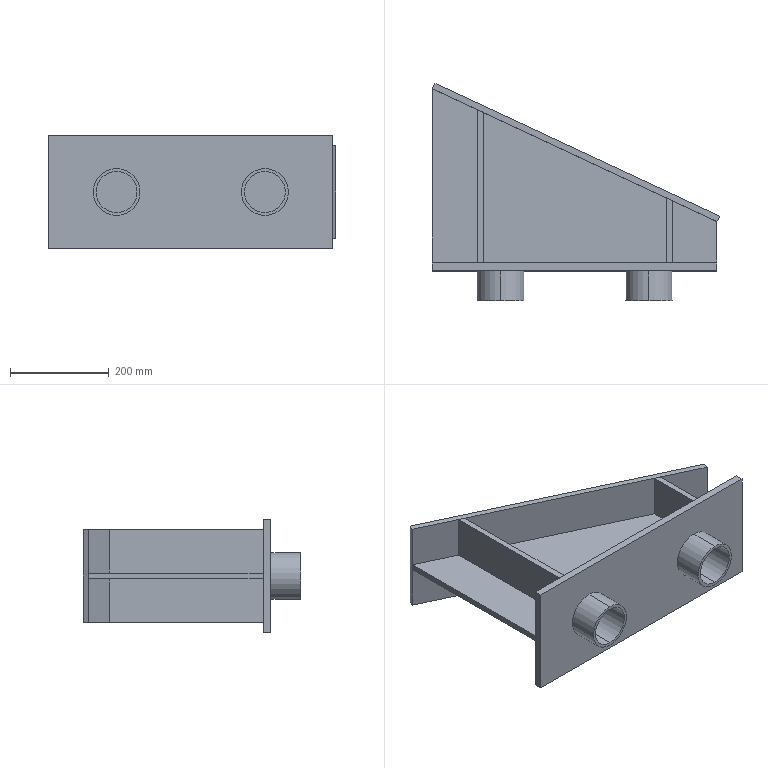Part | STEP file | Spring upper seat (I)_Default<As machined> | 9 solids | 54 faces | box 580.577 x 439.316 x 230 mm | volume 6180967 mm3 | plane 46 | cylinder 8 | commonest cylinder face diameters 83 x4 95 x4